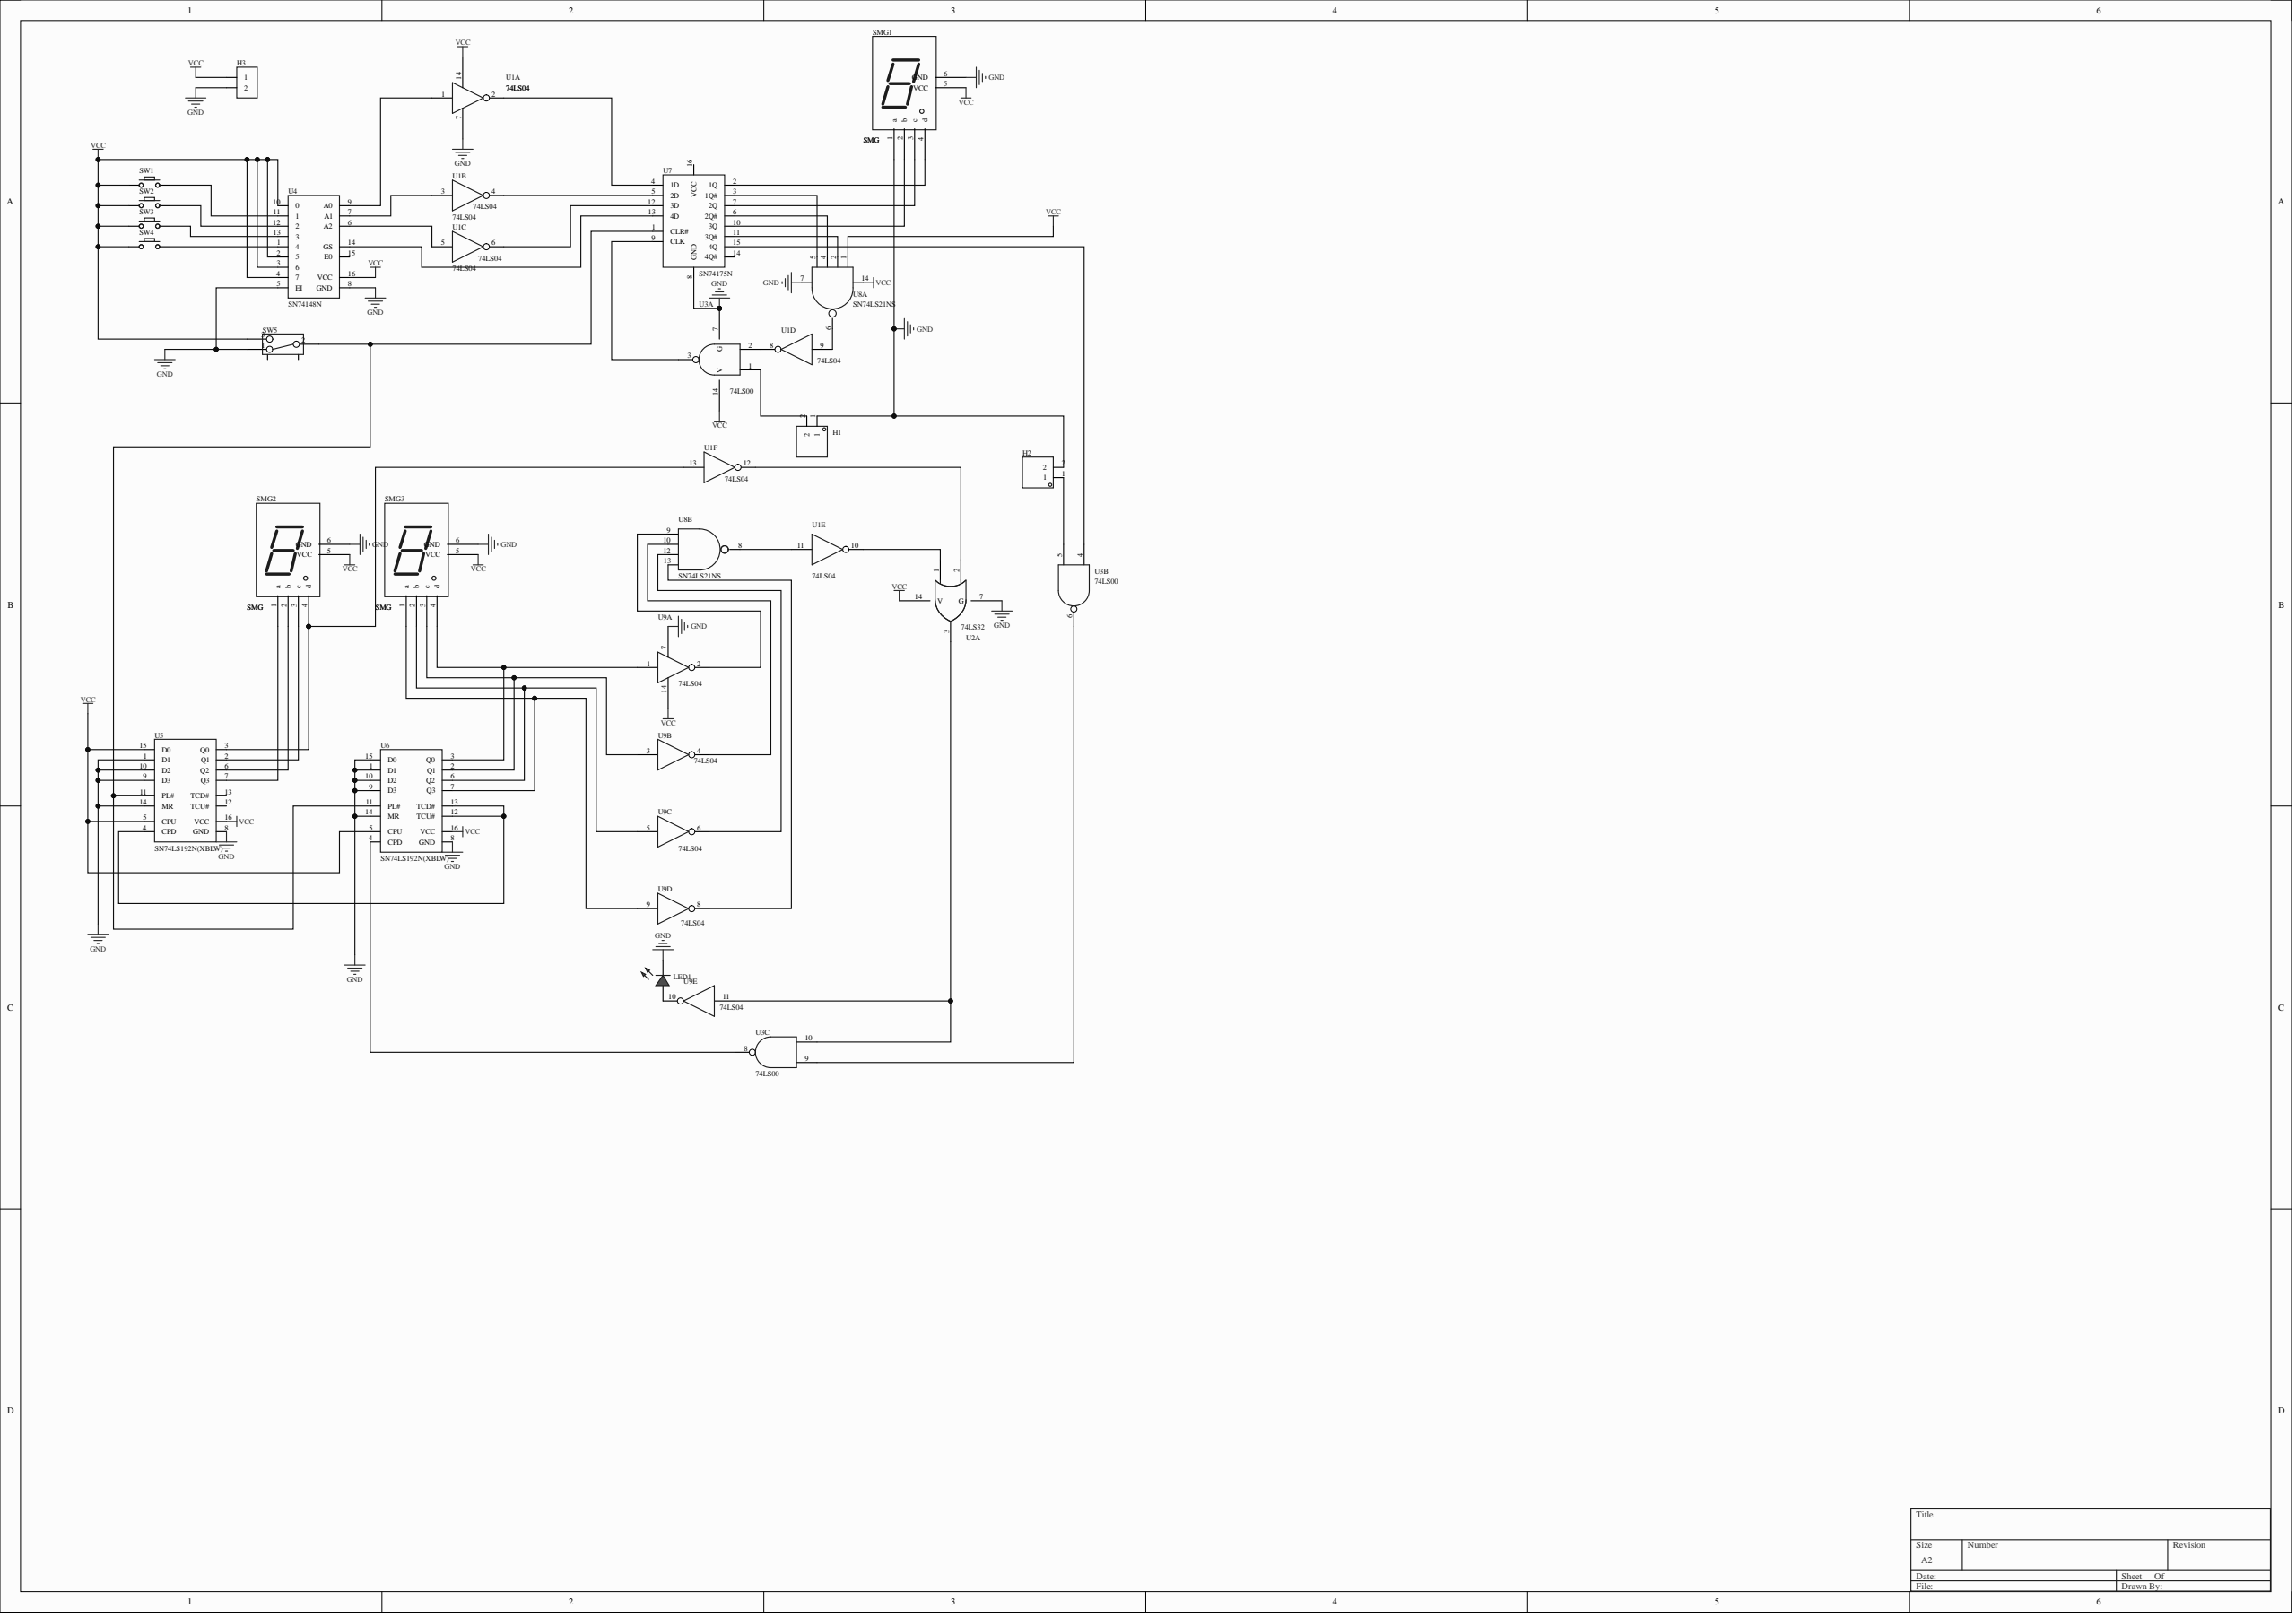Circuit board | Altium Designer | 21 parts | 46 nets
Bill of materials:
Comment,Description,Designator,Footprint,LibRef,Quantity
"","","H1, H2","HDR-TH_2P-P2.54-V-M-1","HDR-M_2.54_1x2P","2"
"","","H3","HDR-TH_2P-P2.54-V-F","HDR-F_2.54_1x2P","1"
"","","LED1","LED_TH-3mm","LED_TH-R_3mm","1"
"SMG","","SMG1, SMG2, SMG3","B含CD译码器的数码管","SMG","3"
"","","SW1, SW2, SW3, SW4","Key_TH_3.5x6x4.3","Key_TH_3.5x6x4.3","4"
"","","SW5","拨动开关","拨动开关_正","1"
"74LS04","","U1, U9","DIP-014","74LS04","2"
"74LS32","","U2","DIP-014","74LS32","1"
"74LS00","","U3","DIP-014","74LS00","1"
"SN74148N","","U4","PDIP-16_L19.3-W6.4-P2.54-LS7.9-BL","SN74148N","1"
"SN74LS192N(XBLW)","Operating voltage:2V~6V; Element count:1; Trigger edge:rising edge; Count rate:40MHz;","U5, U6","PDIP-16_L19.3-W6.4-P2.54-LS7.94-BL","SN74LS192N(XBLW)","2"
"SN74175N","","U7","DIP-16_L19.3-W6.4-P2.54-LS7.6-BL","SN74175N","1"
"SN74LS21NS","Logic type:AND gate; Channels:2; Supply voltage:4.75V~5.25V; Max propagation delay:20ns@5V,15pF;","U8","SOIC-14_L10.0-W5.5-P1.27-LS7.8-BL","SN74LS21NS","1"
Netlist (Protel format):
[
H1
HDR-TH_2P-P2.54-V-M-1




]
[
H2
HDR-TH_2P-P2.54-V-M-1




]
[
H3
HDR-TH_2P-P2.54-V-F




]
[
LED1
LED_TH-3mm




]
[
SMG1
B含CD译码器的数码管
SMG



]
[
SMG2
B含CD译码器的数码管
SMG



]
[
SMG3
B含CD译码器的数码管
SMG



]
[
SW1
Key_TH_3.5x6x4.3




]
[
SW2
Key_TH_3.5x6x4.3




]
[
SW3
Key_TH_3.5x6x4.3




]
[
SW4
Key_TH_3.5x6x4.3




]
[
SW5
拨动开关




]
[
U1
DIP-014
74LS04



]
[
U2
DIP-014
74LS32



]
[
U3
DIP-014
74LS00



]
[
U4
PDIP-16_L19.3-W6.4-P2.54-LS7.9-BL
SN74148N



]
[
U5
PDIP-16_L19.3-W6.4-P2.54-LS7.94-BL
SN74LS192N(XBLW)



]
[
U6
PDIP-16_L19.3-W6.4-P2.54-LS7.94-BL
SN74LS192N(XBLW)



]
[
U7
DIP-16_L19.3-W6.4-P2.54-LS7.6-BL
SN74175N



]
[
U8
SOIC-14_L10.0-W5.5-P1.27-LS7.8-BL
SN74LS21NS



]
[
U9
DIP-014
74LS04



]
(
VCC
H3-1
SMG1-5
SMG2-5
SMG3-5
SW1-A
SW2-A
SW3-A
SW4-A
SW5-3
U1-14
U2-14
U3-14
U4-2
U4-3
U4-4
U4-10
U4-16
U5-5
U5-15
U5-16
U6-5
U6-16
U8-1
U8-14
U9-14
)
(
NetU8_13
U8-13
U9-8
)
(
NetU8_12
U8-12
U9-6
)
(
NetU8_10
U8-10
U9-4
)
(
NetU8_9
U8-9
U9-2
)
(
NetU7_11
U7-11
U8-2
)
(
NetU7_6
U7-6
U8-4
)
(
NetU7_3
U7-3
U8-5
)
(
NetU5_4
U5-4
U6-12
U6-13
)
(
NetU4_14
U4-14
U7-13
)
(
NetU3_8
U3-8
U6-4
)
(
NetU3_6
U3-6
U3-9
)
(
NetU3_4
U3-4
U7-15
)
(
NetU3_3
U3-3
U7-9
)
(
NetU2_3
U2-3
U3-10
U9-11
)
(
NetU1_12
U1-12
U2-2
)
(
NetU1_11
U1-11
U8-8
)
(
NetU1_10
U1-10
U2-1
)
(
NetU1_9
U1-9
U8-6
)
(
NetU1_8
U1-8
U3-2
)
(
NetU1_6
U1-6
U7-12
)
(
NetU1_5
U1-5
U4-6
)
(
NetU1_4
U1-4
U7-5
)
(
NetU1_3
U1-3
U4-7
)
(
NetU1_2
U1-2
U7-4
)
(
NetU1_1
U1-1
U4-9
)
(
NetSW5_2
SW5-2
U5-11
U6-11
U7-1
)
(
NetSW4_B
SW4-B
U4-1
)
(
NetSW3_B
SW3-B
U4-13
)
(
NetSW2_B
SW2-B
U4-12
)
(
NetSW1_B
SW1-B
U4-11
)
(
NetSMG3_4
SMG3-4
U6-3
U9-1
)
(
NetSMG3_3
SMG3-3
U6-2
U9-3
)
(
NetSMG3_2
SMG3-2
U6-6
U9-5
)
(
NetSMG3_1
SMG3-1
U6-7
U9-9
)
(
NetSMG2_4
SMG2-4
U1-13
U5-3
)
(
NetSMG2_3
SMG2-3
U5-2
)
(
NetSMG2_2
SMG2-2
U5-6
)
(
NetSMG2_1
SMG2-1
U5-7
)
(
NetSMG1_4
SMG1-4
U7-2
)
(
NetSMG1_3
SMG1-3
U7-7
)
(
NetSMG1_2
SMG1-2
U7-10
)
(
NetLED1_1
LED1-1
U9-10
)
(
NetH2_1
H2-1
U3-5
)
(
NetH1_2
H1-2
U3-1
)
(
GND
H1-1
H2-2
H3-2
LED1-2
SMG1-1
SMG1-6
SMG2-6
SMG3-6
SW5-1
U1-7
U2-7
U3-7
U4-5
U4-8
U5-1
U5-8
U5-9
U5-10
U5-14
U6-1
U6-8
U6-9
U6-10
U6-14
U6-15
U7-8
U8-7
U9-7
)